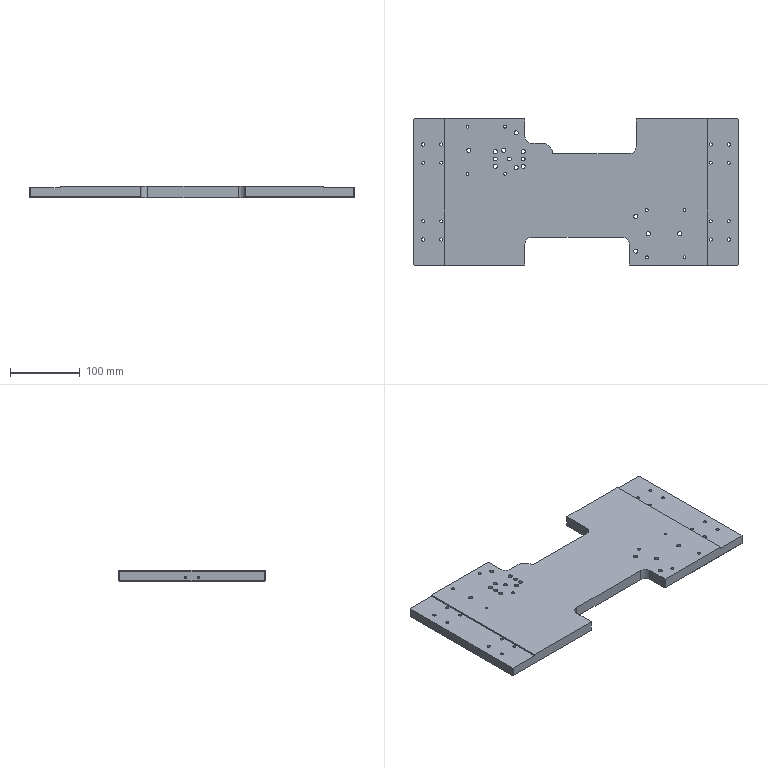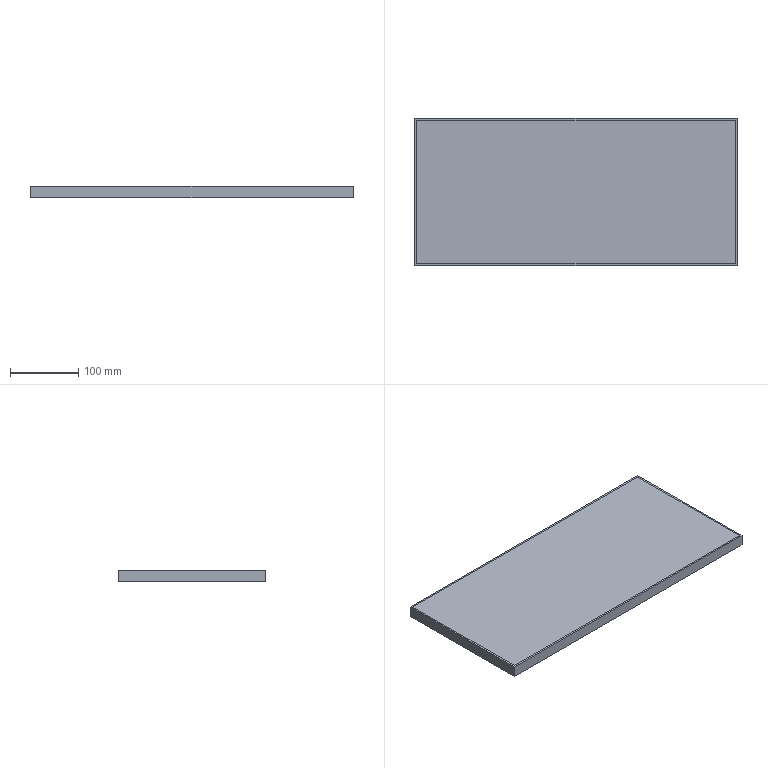CAM job | NX | 3-axis milling, drilling | part box 467 x 210 x 16 mm | stock box 473 x 216 x 17 mm
Tools:
number,name,description,diameter,corner_radius,flute_length,length,flutes
7,D6A45,Milling Tool-5 Parameters,6.0,0.0,3.0,3.0,2
19,4.5ZT,Drilling Tool,4.5,0.0,35.0,50.0,2
1,D63,Milling Tool-5 Parameters,63.0,0.0,50.0,75.0,2
18,5.8ZT,Drilling Tool,5.8,0.0,35.0,50.0,2
20,6.0JD,Milling Tool-5 Parameters,6.0,0.0,30.0,30.0,4
12,5.5ZT,Drilling Tool,5.5,0.0,35.0,50.0,2
14,4.2ZT,Drilling Tool,4.2,0.0,35.0,50.0,2
15,M5,Milling Tool-5 Parameters,4.2,0.0,30.0,30.0,4
13,3.3ZT,Drilling Tool,3.3,0.0,35.0,50.0,2
17,M4,Milling Tool-5 Parameters,3.3,0.0,30.0,30.0,4
10,D10,Milling Tool-5 Parameters,10.0,0.0,50.0,75.0,2
6,D6,Milling Tool-5 Parameters,6.0,0.0,50.0,75.0,2
11,D10JING,Milling Tool-5 Parameters,10.0,0.0,50.0,75.0,2
Operations:
program,operation,operation_type,tool,method,geometry_group,spindle_rpm,surface_speed,feed_per_tooth,feed_cut,feed_plunge,cut_length_mm,path_length_mm,cut_time_min,machine_time_min
PN_0001_AB_GLUE,FLOOR_WALL,VolumeBased25DMillingOperation,D63,METHOD,A,6500.0,1286.0,0.0962,1250.0,100.0,4490.797,4544.797,3.593,3.598
PN_0001_AB_GLUE,DRILLING_COPY_1,Operation,D6A45,METHOD,A,3000.0,56.0,0.0333,200.0,0.0,249.9,2230.659,1.25,1.448
PN_0001_AB_GLUE,DRILLING_COPY_1_COPY_COPY_COPY_COPY,Operation,4.5ZT,METHOD,A,2000.0,20.0,0.0375,150.0,0.0,301.631,1578.65,2.011,2.139
PN_0001_AB_GLUE,DRILLING_COPY_1_COPY_COPY_1,Operation,5.8ZT,METHOD,A,2000.0,18.0,0.03,120.0,0.0,266.91,1104.318,2.224,2.308
PN_0001_AB_GLUE,DRILLING_COPY_1_COPY_COPY_1_COPY,Operation,6.0JD,METHOD,A,1000.0,9.0,0.01,40.0,0.0,234.0,1038.498,5.85,5.93
PN_0001_AB_GLUE,DRILLING_COPY_1_COPY_COPY_1_COPY_1,Operation,5.5ZT,METHOD,A,2000.0,18.0,0.03,120.0,0.0,66.457,239.362,0.5538,0.5711
PN_0001_AB_GLUE,DRILLING_COPY_1_COPY,Operation,4.2ZT,METHOD,A,2000.0,15.0,0.0375,150.0,0.0,174.095,992.199,1.161,1.242
PN_0001_AB_GLUE,DRILLING_COPY_1_COPY_COPY,Operation,M5,METHOD,A,200.0,2.0,0.2,160.0,0.0,156.0,956.01,0.975,1.055
PN_0001_AB_GLUE,DRILLING_COPY_1_COPY_COPY_COPY_COPY_COPY,Operation,3.3ZT,METHOD,A,2000.0,20.0,0.0375,150.0,0.0,132.914,959.962,0.8861,0.9688
PN_0001_AB_GLUE,DRILLING_COPY_1_COPY_COPY_COPY_COPY_COPY_COPY,Operation,M4,METHOD,A,200.0,2.0,0.175,140.0,0.0,100.0,894.134,0.7143,0.7937
PN_0001_AB_GLUE,ZLEVEL_PROFILE,ZLevelMilling,D10,METHOD,A,7000.0,219.0,0.2143,3000.0,1000.0,24719.613,24792.013,8.271,8.278
PN_0001_AB_GLUE,HOLE_MILLING,CylinderMilling,D6,METHOD,A,7000.0,131.0,0.1071,1500.0,100.0,1565.407,3662.448,1.044,1.253
PN_0001_AB_GLUE,ZLEVEL_PROFILE_COPY_1_COPY_COPY_COPY_COPY_2_COPY,ZLevelMilling,D6A45,METHOD,A,7000.0,131.0,0.0714,1000.0,1000.0,2154.922,13052.752,2.155,3.245
PN_0001_AB_GLUE,ZLEVEL_PROFILE_COPY_1,ZLevelMilling,D10JING,METHOD,A,7000.0,219.0,0.0714,1000.0,1000.0,4655.873,4744.623,4.656,4.665
PN_0002_AB_GLUE,FLOOR_WALL_COPY,VolumeBased25DMillingOperation,D63,METHOD,B,6500.0,1286.0,0.0962,1250.0,100.0,3906.797,3960.797,3.125,3.131
PN_0002_AB_GLUE,CUTTER_COMP_11_COPY,VolumeBased25DMillingOperation,D10,METHOD,B,7000.0,219.0,0.1429,2000.0,100.0,7684.993,8941.441,3.842,4.012
PN_0002_AB_GLUE,FLOOR_WALL_1_COPY_1,VolumeBased25DMillingOperation,D10JING,METHOD,B,7000.0,87.0,0.0714,1000.0,100.0,4943.63,5508.628,4.944,5
PN_0002_AB_GLUE,ZLEVEL_PROFILE_COPY_1_COPY_COPY_COPY_COPY_2_COPY_1,ZLevelMilling,D6A45,METHOD,B,7000.0,131.0,0.0714,1000.0,1000.0,1649.968,6112.638,1.65,2.096
PN_0002_AB_GLUE,ZLEVEL_PROFILE_COPY_1_COPY_COPY_COPY_COPY_2_COPY_1_COPY,ZLevelMilling,D6A45,METHOD,B,7000.0,131.0,0.0714,1000.0,1000.0,739.338,5191.745,0.7393,1.185